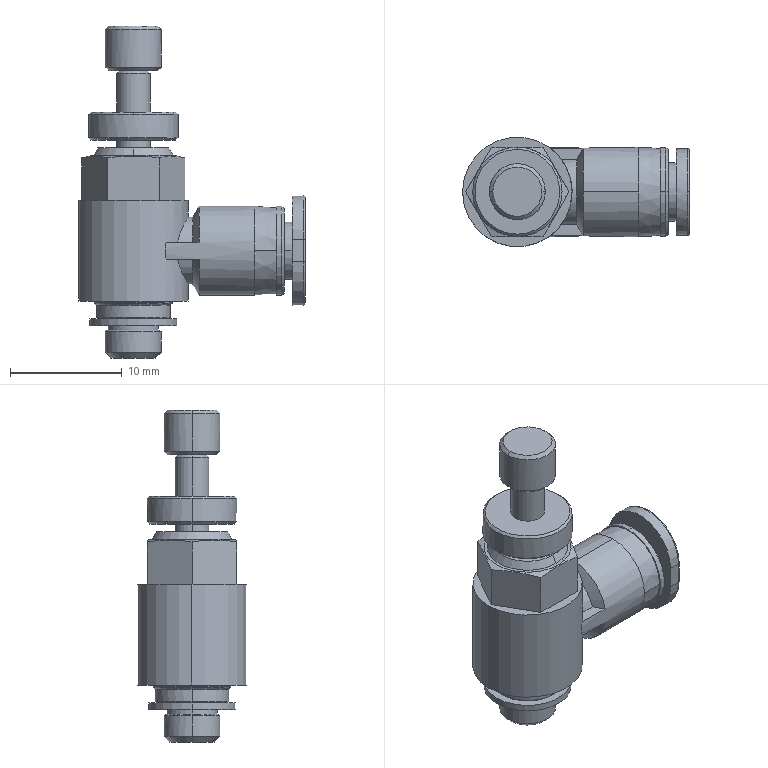Part | NX | 1 solid | 98 faces | box 20.3 x 9.8 x 29.711 mm | volume 1675 mm3 | cylinder 36 | plane 29 | cone 28 | torus 5 | commonest cylinder face diameters 8 x6 3 x4 5 x4 6.6 x4 7.8 x4 0.4 x2